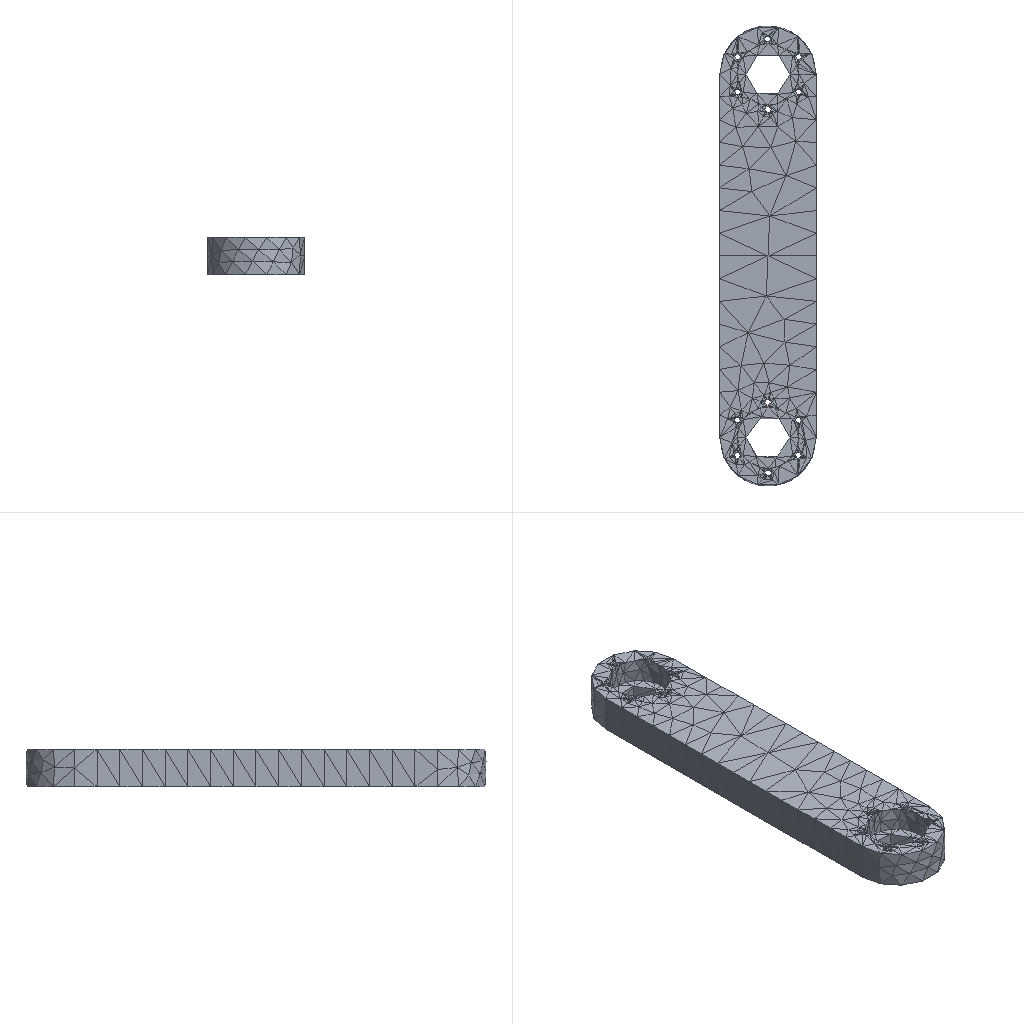Simulation study | ansys workbench
Ansys APDL input file, long lists of numbers shortened:
/batch
/config,noeldb,1     ! force off writing results to database
*get,_wallstrt,active,,time,wall
! ANSYS input file written by Workbench version 2022 R1
! File used for geometry attach:
/title,111--____ (D5)
! ****** Begin Custom Load Command Snippet ******
/COM, ACT Extensions:
/COM,     LSDYNA, 2021.1
/COM,
! ****** End   Custom Load Command Snippet ******
*DIM,_wb_ProjectScratch_dir,string,248
_wb_ProjectScratch_dir(1) = ''
*DIM,_wb_SolverFiles_dir,string,248
_wb_SolverFiles_dir(1) = ''
*DIM,_wb_userfiles_dir,string,248
_wb_userfiles_dir(1) = ''
/com,--- Data in consistent NMM units. See Solving Units in the help system for more information.
/units,MPA
/nopr
/wb,file,start              !  signify a WB generated input file
/prep7
! Turn off shape checking because checks already performed inside WB mesher.
! See help system for more information.
SHPP,OFF,,NOWARN
/nolist
etcon,set             ! allow ANSYS to choose best KEYOP's for 180x elements, resets any applicable keyopt to MAPDL defaults
/com,*********** Nodes for the whole assembly ***********
nblock,3,,8621
(1i9,3e20.9e3)
        1     1.611560527E+01    -9.336711199E+01     1.672729262E+01
! (7837 more lines like these left out)
-1
/wb,elem,start            !  set before creation of elements
/com,*********** Elements for Body 1 "6__4-FreeParts|__(__)4" ***********
et,1,187
eblock,19,solid,,4180
(19i9)
        1        1        1        1        0        0        0        0       10        0        1      662     1273     1276     1275     5475     7837     5477     5476
! (8359 more lines like these left out)
-1
/wb,elem,end               !  done creating elements
/com,*********** Send User Defined Coordinate System(s) ***********
csys,0
toffst,273.15,  ! Temperature offset from absolute zero
/com,*********** Set Reference Temperature ***********
tref,22.
/wb,mat,start              !  starting to send materials
/com,*********** Send Materials ***********
Temperature = 'TEMP' ! Temperature
MP,DENS,1,7.85e-09,	! tonne mm^-3
MP,ALPX,1,1.2e-05,	! C^-1
MP,C,1,434000000,	! mm^2 s^-2 C^-1
MP,KXX,1,60.5,	! tonne mm s^-3 C^-1
MP,RSVX,1,0.00017,	! ohm mm
MP,EX,1,200000,	! tonne s^-2 mm^-1
MP,NUXY,1,0.3,
MP,MURX,1,10000,
/wb,mat,end                !  done sending materials
!************************* Model Summary ********************
!6__4-FreeParts|__(__)4,	结构钢,	matid,	1
!************************* End Model Summary ********************
! get the diagonal of the bounding box. Needed later for other things
*get,_xmin,node,,mnloc,x
*get,_ymin,node,,mnloc,y
*get,_zmin,node,,mnloc,z
*get,_xmax,node,,mxloc,x
*get,_ymax,node,,mxloc,y
*get,_zmax,node,,mxloc,z
_ASMDIAG=(_xmax-_xmin)*(_xmax-_xmin)+(_ymax-_ymin)*(_ymax-_ymin)+(_zmax-_zmin)*(_zmax-_zmin)
_ASMDIAG=SQRT(_ASMDIAG)
/wb,contact,start          !  starting to send contact
/wb,contact,end            !  done creating contacts
/com,*********** Send Named Selection as Node Component ***********
CMBLOCK,______  ,NODE,     2081
(8i10)
         1         2         3         4        10        11        12        13
! (260 more lines like these left out)
/golist
/wb,load,start             !  starting to send loads
/com,*********** Fixed Supports ***********
CMBLOCK,_FIXEDSU,NODE,     2081
(8i10)
         1         2         3         4        10        11        12        13
! (260 more lines like these left out)
cmsel,s,_FIXEDSU
d,all,all
nsel,all
/com,*********** Define Force Using Surface Effect Elements ***********
local,12,0,0.,0.,0.,0.,0.,0.
csys,0
et,2,154
eblock,10,,,470
(15i9)
     6335        2        2        2       12      441      732      490      490     4431     4657      490     4430
! (469 more lines like these left out)
-1
esel,s,type,,2
keyop,2,2,1                ! Apply load in local coordinate system
keyop,2,7,1                ! Use original area so load is constant in large deformation
esel,all
/gst,on,on
fini
*get,_numnode,node,0,count
*get,_numelem,elem,0,count
*get, _MAXELEMNUM, elem, 0, NUM, MAX
*get, _MAXNODENUM, node, 0, NUM, MAX
*get, _MAXELEMTYPE, etyp, 0, NUM, MAX
*get, _MAXREALCONST, real, 0, NUM, MAX
/go
/wb,load,end               !  done creating loads
/com,--- Number of total nodes = %_numnode%
/com,--- Number of contact elements = 470
/com,--- Number of spring elements = 0
/com,--- Number of bearing elements = 0
/com,--- Number of solid elements = 4180
/com,--- Number of condensed parts = 0
/com,--- Number of total elements = %_numelem%
*get,_wallbsol,active,,time,wall
/com,****************************************************************************
/com,*************************    SOLUTION       ********************************
/com,****************************************************************************
/solu
antype,0                   ! static analysis
_thickRatio=  1     ! Ratio of thick parts in the model
eqsl,pcg,1e-8,,,,,,1
cntr,print,1               ! print out contact info and also make no initial contact an error
dmpoption,emat,no             ! Don't combine emat file for DANSYS
dmpoption,esav,no             ! Don't combine esav file for DANSYS
nldiag,cont,iter           ! print out contact info each equilibrium iteration
rescontrol,,none                 ! Do not keep any restart files
/com,****************************************************
/com,******************* SOLVE FOR LS 1 OF 1 ****************
esel,s,type,,2
nsle
sfe,all,1,pres,1,0.
sfe,all,2,pres,1,0.
sfe,all,3,pres,1,-0.6729
nsel,all
esel,all
/nopr
/gopr
nsub,1,1,1
time,1.
outres,erase
outres,all,none
outres,nsol,all,
outres,rsol,all
outres,eangl,all
outres,etmp,all
outres,veng,all
outres,strs,all,
outres,epel,all,
outres,eppl,all,
outres,cont,all,
! *********** WB SOLVE COMMAND ***********
! check interactive state
*get,ANSINTER_,active,,int
*if,ANSINTER_,ne,0,then
/eof
*endif
solve
/com *************** Write FE CONNECTORS *********
CEWRITE,file,ce,,INTE
/com,****************************************************
/com,*************** FINISHED SOLVE FOR LS 1 *************
*get,_wallasol,active,,time,wall
/nopr
*get,_numnode,node,0,count
*get,_numelem,elem,0,count
*get, _MAXELEMNUM, elem, 0, NUM, MAX
*get, _MAXNODENUM, node, 0, NUM, MAX,,,INTERNAL
*get, _MAXELEMTYPE, etyp, 0, NUM, MAX
*get, _MAXREALCONST, real, 0, NUM, MAX
/gopr
*get,_PCGITER,active,,solu,cgiter
/post1
xmlo,ENCODING,ISO-8859-1
xmlo,parm
/xml,parm,xml
fini
/gopr
*get,_walldone,active,,time,wall
_preptime=(_wallbsol-_wallstrt)*3600
_solvtime=(_wallasol-_wallbsol)*3600
_posttime=(_walldone-_wallasol)*3600
_totaltim=(_walldone-_wallstrt)*3600
*get,_dlbratio,active,0,solu,dlbr
*get,_combtime,active,0,solu,comb
*get,_ssmode,active,0,solu,ssmm
*get,_ndofs,active,0,solu,ndof
*get,_sol_end_time,active,0,set,time
*if,_sol_end_time,eq,1.,then
/fclean				!clean distributed files
*endif
/com,--- Total number of nodes = %_numnode%
/com,--- Total number of elements = %_numelem%
/com,--- Element load balance ratio = %_dlbratio%
/com,--- Time to combine distributed files = %_combtime%
/com,--- Sparse memory mode = %_ssmode%
/com,--- Number of DOF = %_ndofs%
/wb,file,end               ! done with WB generated input